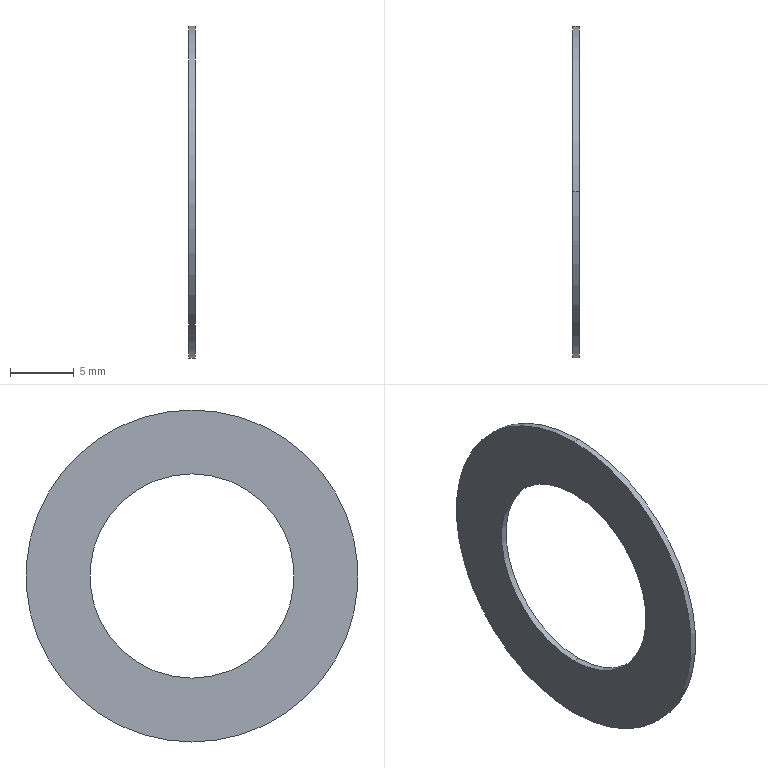Part | SolidWorks | features Extrusion 1 | 1 solid | 6 faces | box 0.5 x 26 x 26 mm | volume 164.934 mm3 | cylinder 4 | plane 2 | commonest cylinder face diameters 16 x2 26 x2
STEP:
#1=CARTESIAN_POINT('',(0.5,0.,8.));
#2=VERTEX_POINT('',#1);
#3=CARTESIAN_POINT('',(0.5,0.,-8.));
#4=VERTEX_POINT('',#3);
#5=CARTESIAN_POINT('',(0.5,0.,0.));
#6=DIRECTION('',(1.,0.,0.));
#7=DIRECTION('',(0.,0.,-1.));
#8=AXIS2_PLACEMENT_3D('',#5,#6,#7);
#9=CIRCLE('',#8,8.);
#10=EDGE_CURVE('',#2,#4,#9,.T.);
#11=ORIENTED_EDGE('',*,*,#10,.T.);
#12=CARTESIAN_POINT('',(0.,0.,-8.));
#13=VERTEX_POINT('',#12);
#14=CARTESIAN_POINT('',(0.5,0.,-8.));
#15=DIRECTION('',(-1.,0.,0.));
#16=VECTOR('',#15,1000.);
#17=LINE('',#14,#16);
#18=EDGE_CURVE('',#4,#13,#17,.T.);
#19=ORIENTED_EDGE('',*,*,#18,.T.);
#20=CARTESIAN_POINT('',(0.,0.,8.));
#21=VERTEX_POINT('',#20);
#22=CARTESIAN_POINT('',(0.,0.,0.));
#23=DIRECTION('',(1.,0.,0.));
#24=DIRECTION('',(0.,0.,-1.));
#25=AXIS2_PLACEMENT_3D('',#22,#23,#24);
#26=CIRCLE('',#25,8.);
#27=EDGE_CURVE('',#21,#13,#26,.T.);
#28=ORIENTED_EDGE('',*,*,#27,.F.);
#29=CARTESIAN_POINT('',(0.5,0.,8.));
#30=DIRECTION('',(-1.,0.,0.));
#31=VECTOR('',#30,1000.);
#32=LINE('',#29,#31);
#33=EDGE_CURVE('',#2,#21,#32,.T.);
#34=ORIENTED_EDGE('',*,*,#33,.F.);
#35=EDGE_LOOP('',(#11,#19,#28,#34));
#36=FACE_OUTER_BOUND('',#35,.T.);
#37=CARTESIAN_POINT('',(0.5,0.,0.));
#38=DIRECTION('',(-1.,0.,0.));
#39=DIRECTION('',(0.,0.,1.));
#40=AXIS2_PLACEMENT_3D('',#37,#38,#39);
#41=CYLINDRICAL_SURFACE('',#40,8.);
#42=ADVANCED_FACE('',(#36),#41,.F.);
#43=CARTESIAN_POINT('',(0.5,0.,-13.));
#44=VERTEX_POINT('',#43);
#45=CARTESIAN_POINT('',(0.5,0.,13.));
#46=VERTEX_POINT('',#45);
#47=CARTESIAN_POINT('',(0.5,0.,0.));
#48=DIRECTION('',(1.,0.,0.));
#49=DIRECTION('',(0.,0.,-1.));
#50=AXIS2_PLACEMENT_3D('',#47,#48,#49);
#51=CIRCLE('',#50,13.);
#52=EDGE_CURVE('',#44,#46,#51,.T.);
#53=ORIENTED_EDGE('',*,*,#52,.F.);
#54=CARTESIAN_POINT('',(0.,0.,-13.));
#55=VERTEX_POINT('',#54);
#56=CARTESIAN_POINT('',(0.5,0.,-13.));
#57=DIRECTION('',(-1.,0.,0.));
#58=VECTOR('',#57,1000.);
#59=LINE('',#56,#58);
#60=EDGE_CURVE('',#44,#55,#59,.T.);
#61=ORIENTED_EDGE('',*,*,#60,.T.);
#62=CARTESIAN_POINT('',(0.,0.,13.));
#63=VERTEX_POINT('',#62);
#64=CARTESIAN_POINT('',(0.,0.,0.));
#65=DIRECTION('',(1.,0.,0.));
#66=DIRECTION('',(0.,0.,-1.));
#67=AXIS2_PLACEMENT_3D('',#64,#65,#66);
#68=CIRCLE('',#67,13.);
#69=EDGE_CURVE('',#55,#63,#68,.T.);
#70=ORIENTED_EDGE('',*,*,#69,.T.);
#71=CARTESIAN_POINT('',(0.5,0.,13.));
#72=DIRECTION('',(-1.,0.,0.));
#73=VECTOR('',#72,1000.);
#74=LINE('',#71,#73);
#75=EDGE_CURVE('',#46,#63,#74,.T.);
#76=ORIENTED_EDGE('',*,*,#75,.F.);
#77=EDGE_LOOP('',(#53,#61,#70,#76));
#78=FACE_OUTER_BOUND('',#77,.T.);
#79=CARTESIAN_POINT('',(0.5,0.,0.));
#80=DIRECTION('',(-1.,0.,0.));
#81=DIRECTION('',(0.,0.,1.));
#82=AXIS2_PLACEMENT_3D('',#79,#80,#81);
#83=CYLINDRICAL_SURFACE('',#82,13.);
#84=ADVANCED_FACE('',(#78),#83,.T.);
#85=CARTESIAN_POINT('',(0.5,0.,0.));
#86=DIRECTION('',(1.,0.,0.));
#87=DIRECTION('',(0.,0.,-1.));
#88=AXIS2_PLACEMENT_3D('',#85,#86,#87);
#89=CIRCLE('',#88,13.);
#90=EDGE_CURVE('',#46,#44,#89,.T.);
#91=ORIENTED_EDGE('',*,*,#90,.T.);
#92=ORIENTED_EDGE('',*,*,#52,.T.);
#93=EDGE_LOOP('',(#91,#92));
#94=FACE_OUTER_BOUND('',#93,.T.);
#95=ORIENTED_EDGE('',*,*,#10,.F.);
#96=CARTESIAN_POINT('',(0.5,0.,0.));
#97=DIRECTION('',(1.,0.,0.));
#98=DIRECTION('',(0.,0.,-1.));
#99=AXIS2_PLACEMENT_3D('',#96,#97,#98);
#100=CIRCLE('',#99,8.);
#101=EDGE_CURVE('',#4,#2,#100,.T.);
#102=ORIENTED_EDGE('',*,*,#101,.F.);
#103=EDGE_LOOP('',(#95,#102));
#104=FACE_BOUND('',#103,.T.);
#105=CARTESIAN_POINT('',(0.5,0.,0.));
#106=DIRECTION('',(1.,0.,0.));
#107=DIRECTION('',(0.,0.,-1.));
#108=AXIS2_PLACEMENT_3D('',#105,#106,#107);
#109=PLANE('',#108);
#110=ADVANCED_FACE('',(#94,#104),#109,.T.);
#111=CARTESIAN_POINT('',(0.,0.,0.));
#112=DIRECTION('',(1.,0.,0.));
#113=DIRECTION('',(0.,0.,-1.));
#114=AXIS2_PLACEMENT_3D('',#111,#112,#113);
#115=CIRCLE('',#114,13.);
#116=EDGE_CURVE('',#63,#55,#115,.T.);
#117=ORIENTED_EDGE('',*,*,#116,.F.);
#118=ORIENTED_EDGE('',*,*,#69,.F.);
#119=EDGE_LOOP('',(#117,#118));
#120=FACE_OUTER_BOUND('',#119,.T.);
#121=ORIENTED_EDGE('',*,*,#27,.T.);
#122=CARTESIAN_POINT('',(0.,0.,0.));
#123=DIRECTION('',(1.,0.,0.));
#124=DIRECTION('',(0.,0.,-1.));
#125=AXIS2_PLACEMENT_3D('',#122,#123,#124);
#126=CIRCLE('',#125,8.);
#127=EDGE_CURVE('',#13,#21,#126,.T.);
#128=ORIENTED_EDGE('',*,*,#127,.T.);
#129=EDGE_LOOP('',(#121,#128));
#130=FACE_BOUND('',#129,.T.);
#131=CARTESIAN_POINT('',(0.,0.,0.));
#132=DIRECTION('',(1.,0.,0.));
#133=DIRECTION('',(0.,0.,-1.));
#134=AXIS2_PLACEMENT_3D('',#131,#132,#133);
#135=PLANE('',#134);
#136=ADVANCED_FACE('',(#120,#130),#135,.F.);
#137=ORIENTED_EDGE('',*,*,#60,.F.);
#138=ORIENTED_EDGE('',*,*,#90,.F.);
#139=ORIENTED_EDGE('',*,*,#75,.T.);
#140=ORIENTED_EDGE('',*,*,#116,.T.);
#141=EDGE_LOOP('',(#137,#138,#139,#140));
#142=FACE_OUTER_BOUND('',#141,.T.);
#143=CARTESIAN_POINT('',(0.5,0.,0.));
#144=DIRECTION('',(-1.,0.,0.));
#145=DIRECTION('',(0.,0.,1.));
#146=AXIS2_PLACEMENT_3D('',#143,#144,#145);
#147=CYLINDRICAL_SURFACE('',#146,13.);
#148=ADVANCED_FACE('',(#142),#147,.T.);
#149=ORIENTED_EDGE('',*,*,#18,.F.);
#150=ORIENTED_EDGE('',*,*,#101,.T.);
#151=ORIENTED_EDGE('',*,*,#33,.T.);
#152=ORIENTED_EDGE('',*,*,#127,.F.);
#153=EDGE_LOOP('',(#149,#150,#151,#152));
#154=FACE_OUTER_BOUND('',#153,.T.);
#155=CARTESIAN_POINT('',(0.5,0.,0.));
#156=DIRECTION('',(-1.,0.,0.));
#157=DIRECTION('',(0.,0.,1.));
#158=AXIS2_PLACEMENT_3D('',#155,#156,#157);
#159=CYLINDRICAL_SURFACE('',#158,8.);
#160=ADVANCED_FACE('',(#154),#159,.F.);
#161=CLOSED_SHELL('',(#42,#84,#110,#136,#148,#160));
#162=MANIFOLD_SOLID_BREP('',#161);
#163=CARTESIAN_POINT('',(0.,0.,0.));
#164=DIRECTION('',(0.,0.,1.));
#165=DIRECTION('',(1.,0.,0.));
#166=AXIS2_PLACEMENT_3D('',#163,#164,#165);
#167=(LENGTH_UNIT()NAMED_UNIT(*)SI_UNIT(.MILLI.,.METRE.));
#168=UNCERTAINTY_MEASURE_WITH_UNIT(LENGTH_MEASURE(0.00001),#167,'','');
#169=(NAMED_UNIT(*)PLANE_ANGLE_UNIT()SI_UNIT($,.RADIAN.));
#170=(NAMED_UNIT(*)SI_UNIT($,.STERADIAN.)SOLID_ANGLE_UNIT());
#171=(GEOMETRIC_REPRESENTATION_CONTEXT(3)GLOBAL_UNCERTAINTY_ASSIGNED_CONTEXT((#168))GLOBAL_UNIT_ASSIGNED_CONTEXT((#167,#169,#170))REPRESENTATION_CONTEXT('',''));
#172=ADVANCED_BREP_SHAPE_REPRESENTATION('',(#162,#166),#171);